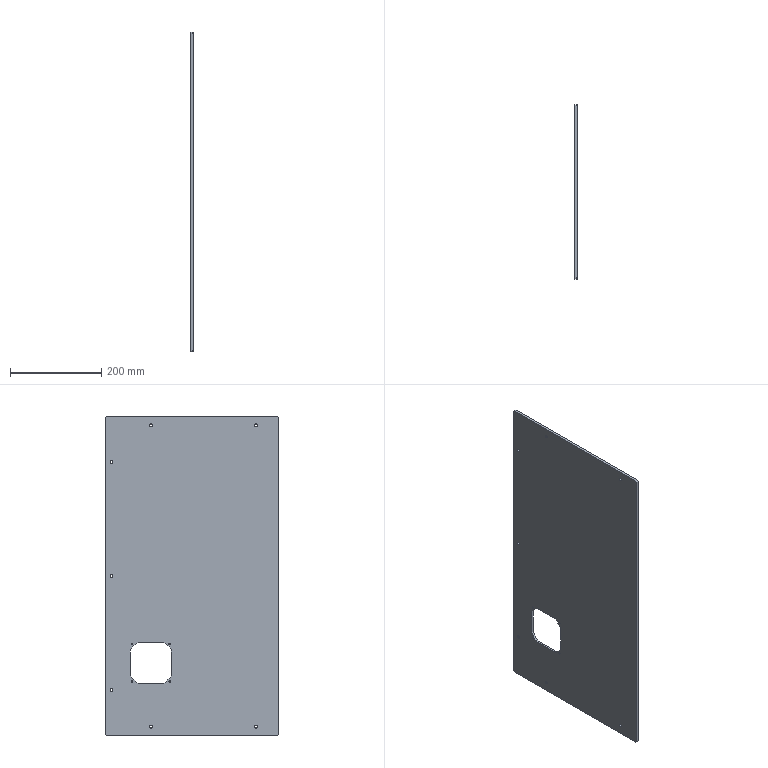Part | STEP file | 227H056124 Rear Cover SLDPRT_Default | 1 solid | 40 faces | box 5 x 380 x 700 mm | volume 1290724 mm3 | cylinder 26 | plane 14 | commonest cylinder face diameters 6 x14 3.5 x8 106 x4